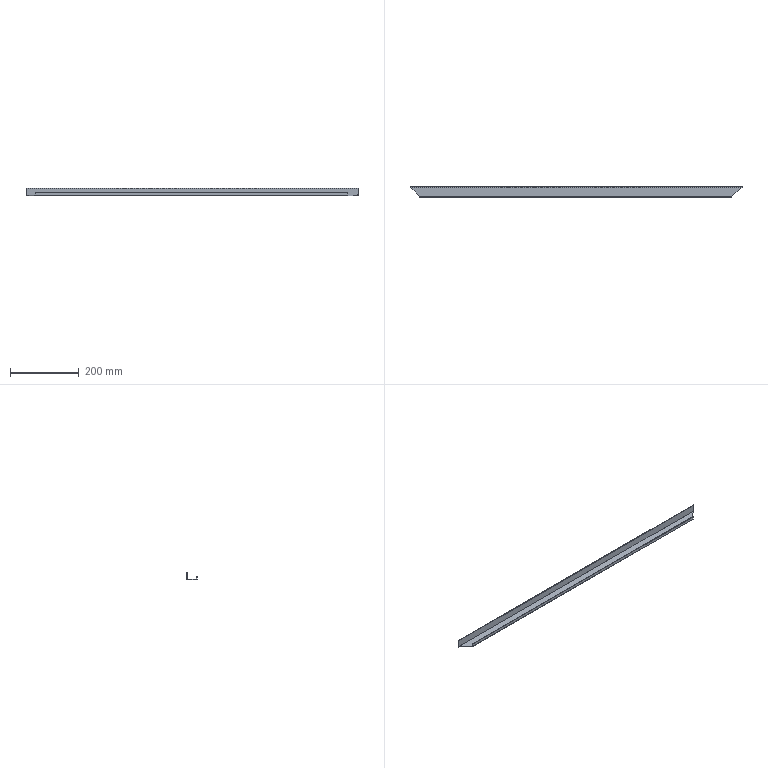Part | STEP file | Rear Closing Plate Door Frame Upper | 1 solid | 34 faces | box 963 x 30 x 22 mm | volume 107174 mm3 | plane 22 | cylinder 10 | spline 2 | commonest cylinder face diameters 0.2 x8 4.2 x2
STEP:
#1=CARTESIAN_POINT('',(-1.351,217.392,2.4));
#2=VERTEX_POINT('',#1);
#3=CARTESIAN_POINT('',(-1.251,217.392,2.3));
#4=VERTEX_POINT('',#3);
#5=CARTESIAN_POINT('',(-1.351,217.392,2.3));
#6=DIRECTION('',(0.,1.,0.));
#7=DIRECTION('',(0.,0.,1.));
#8=AXIS2_PLACEMENT_3D('',#5,#6,#7);
#9=CIRCLE('',#8,0.1);
#10=EDGE_CURVE('',#2,#4,#9,.T.);
#11=ORIENTED_EDGE('',*,*,#10,.F.);
#12=CARTESIAN_POINT('',(-1.351,219.392,2.4));
#13=VERTEX_POINT('',#12);
#14=CARTESIAN_POINT('',(-1.351,-1707.111,2.4));
#15=DIRECTION('',(0.,1.,0.));
#16=VECTOR('',#15,1000.);
#17=LINE('',#14,#16);
#18=EDGE_CURVE('',#2,#13,#17,.T.);
#19=ORIENTED_EDGE('',*,*,#18,.T.);
#20=CARTESIAN_POINT('',(-1.251,219.392,2.3));
#21=VERTEX_POINT('',#20);
#22=CARTESIAN_POINT('',(-1.351,219.392,2.3));
#23=DIRECTION('',(0.,1.,0.));
#24=DIRECTION('',(0.,0.,1.));
#25=AXIS2_PLACEMENT_3D('',#22,#23,#24);
#26=CIRCLE('',#25,0.1);
#27=EDGE_CURVE('',#13,#21,#26,.T.);
#28=ORIENTED_EDGE('',*,*,#27,.T.);
#29=CARTESIAN_POINT('',(-1.251,-1707.111,2.3));
#30=DIRECTION('',(0.,-1.,0.));
#31=VECTOR('',#30,1000.);
#32=LINE('',#29,#31);
#33=EDGE_CURVE('',#21,#4,#32,.T.);
#34=ORIENTED_EDGE('',*,*,#33,.T.);
#35=EDGE_LOOP('',(#11,#19,#28,#34));
#36=FACE_OUTER_BOUND('',#35,.T.);
#37=CARTESIAN_POINT('',(-1.351,-1707.111,2.3));
#38=DIRECTION('',(0.,1.,0.));
#39=DIRECTION('',(0.,0.,1.));
#40=AXIS2_PLACEMENT_3D('',#37,#38,#39);
#41=CYLINDRICAL_SURFACE('',#40,0.1);
#42=ADVANCED_FACE('',(#36),#41,.F.);
#43=CARTESIAN_POINT('',(957.849,217.392,2.4));
#44=VERTEX_POINT('',#43);
#45=CARTESIAN_POINT('',(957.949,217.392,2.3));
#46=VERTEX_POINT('',#45);
#47=CARTESIAN_POINT('',(957.849,217.392,2.3));
#48=DIRECTION('',(0.,1.,0.));
#49=DIRECTION('',(0.,0.,1.));
#50=AXIS2_PLACEMENT_3D('',#47,#48,#49);
#51=CIRCLE('',#50,0.1);
#52=EDGE_CURVE('',#44,#46,#51,.T.);
#53=ORIENTED_EDGE('',*,*,#52,.F.);
#54=CARTESIAN_POINT('',(957.849,219.392,2.4));
#55=VERTEX_POINT('',#54);
#56=CARTESIAN_POINT('',(957.849,-1707.111,2.4));
#57=DIRECTION('',(0.,1.,0.));
#58=VECTOR('',#57,1000.);
#59=LINE('',#56,#58);
#60=EDGE_CURVE('',#44,#55,#59,.T.);
#61=ORIENTED_EDGE('',*,*,#60,.T.);
#62=CARTESIAN_POINT('',(957.949,219.392,2.3));
#63=VERTEX_POINT('',#62);
#64=CARTESIAN_POINT('',(957.849,219.392,2.3));
#65=DIRECTION('',(0.,1.,0.));
#66=DIRECTION('',(0.,0.,1.));
#67=AXIS2_PLACEMENT_3D('',#64,#65,#66);
#68=CIRCLE('',#67,0.1);
#69=EDGE_CURVE('',#55,#63,#68,.T.);
#70=ORIENTED_EDGE('',*,*,#69,.T.);
#71=CARTESIAN_POINT('',(957.949,-1707.111,2.3));
#72=DIRECTION('',(0.,-1.,0.));
#73=VECTOR('',#72,1000.);
#74=LINE('',#71,#73);
#75=EDGE_CURVE('',#63,#46,#74,.T.);
#76=ORIENTED_EDGE('',*,*,#75,.T.);
#77=EDGE_LOOP('',(#53,#61,#70,#76));
#78=FACE_OUTER_BOUND('',#77,.T.);
#79=CARTESIAN_POINT('',(957.849,-1707.111,2.3));
#80=DIRECTION('',(0.,1.,0.));
#81=DIRECTION('',(0.,0.,1.));
#82=AXIS2_PLACEMENT_3D('',#79,#80,#81);
#83=CYLINDRICAL_SURFACE('',#82,0.1);
#84=ADVANCED_FACE('',(#78),#83,.F.);
#85=CARTESIAN_POINT('',(929.749,191.692,2.));
#86=VERTEX_POINT('',#85);
#87=CARTESIAN_POINT('',(929.749,191.492,2.));
#88=VERTEX_POINT('',#87);
#89=CARTESIAN_POINT('',(929.749,0.,2.));
#90=DIRECTION('',(0.,-1.,0.));
#91=VECTOR('',#90,1000.);
#92=LINE('',#89,#91);
#93=EDGE_CURVE('',#86,#88,#92,.T.);
#94=ORIENTED_EDGE('',*,*,#93,.F.);
#95=CARTESIAN_POINT('',(929.949,191.692,2.));
#96=VERTEX_POINT('',#95);
#97=CARTESIAN_POINT('',(929.849,191.692,2.));
#98=DIRECTION('',(0.,0.,-1.));
#99=DIRECTION('',(-1.,0.,0.));
#100=AXIS2_PLACEMENT_3D('',#97,#98,#99);
#101=CIRCLE('',#100,0.1);
#102=EDGE_CURVE('',#86,#96,#101,.T.);
#103=ORIENTED_EDGE('',*,*,#102,.T.);
#104=CARTESIAN_POINT('',(929.949,191.577,2.));
#105=VERTEX_POINT('',#104);
#106=CARTESIAN_POINT('',(929.949,0.,2.));
#107=DIRECTION('',(0.,1.,0.));
#108=VECTOR('',#107,1000.);
#109=LINE('',#106,#108);
#110=EDGE_CURVE('',#105,#96,#109,.T.);
#111=ORIENTED_EDGE('',*,*,#110,.F.);
#112=CARTESIAN_POINT('',(957.641,217.292,2.));
#113=VERTEX_POINT('',#112);
#114=CARTESIAN_POINT('',(957.641,217.292,2.));
#115=DIRECTION('',(-0.7328,-0.6805,0.));
#116=VECTOR('',#115,1000.);
#117=LINE('',#114,#116);
#118=EDGE_CURVE('',#113,#105,#117,.T.);
#119=ORIENTED_EDGE('',*,*,#118,.F.);
#120=CARTESIAN_POINT('',(-1.151,217.292,2.));
#121=VERTEX_POINT('',#120);
#122=CARTESIAN_POINT('',(0.,217.292,2.));
#123=DIRECTION('',(1.,0.,0.));
#124=VECTOR('',#123,1000.);
#125=LINE('',#122,#124);
#126=EDGE_CURVE('',#121,#113,#125,.T.);
#127=ORIENTED_EDGE('',*,*,#126,.F.);
#128=CARTESIAN_POINT('',(24.549,191.592,2.));
#129=VERTEX_POINT('',#128);
#130=CARTESIAN_POINT('',(24.549,191.592,2.));
#131=DIRECTION('',(-0.7071,0.7071,0.));
#132=VECTOR('',#131,1000.);
#133=LINE('',#130,#132);
#134=EDGE_CURVE('',#129,#121,#133,.T.);
#135=ORIENTED_EDGE('',*,*,#134,.F.);
#136=CARTESIAN_POINT('',(24.549,191.692,2.));
#137=VERTEX_POINT('',#136);
#138=CARTESIAN_POINT('',(24.549,0.,2.));
#139=DIRECTION('',(0.,-1.,0.));
#140=VECTOR('',#139,1000.);
#141=LINE('',#138,#140);
#142=EDGE_CURVE('',#137,#129,#141,.T.);
#143=ORIENTED_EDGE('',*,*,#142,.F.);
#144=CARTESIAN_POINT('',(24.749,191.692,2.));
#145=VERTEX_POINT('',#144);
#146=CARTESIAN_POINT('',(24.649,191.692,2.));
#147=DIRECTION('',(0.,0.,-1.));
#148=DIRECTION('',(-1.,0.,0.));
#149=AXIS2_PLACEMENT_3D('',#146,#147,#148);
#150=CIRCLE('',#149,0.1);
#151=EDGE_CURVE('',#137,#145,#150,.T.);
#152=ORIENTED_EDGE('',*,*,#151,.T.);
#153=CARTESIAN_POINT('',(24.749,191.492,2.));
#154=VERTEX_POINT('',#153);
#155=CARTESIAN_POINT('',(24.749,0.,2.));
#156=DIRECTION('',(0.,1.,0.));
#157=VECTOR('',#156,1000.);
#158=LINE('',#155,#157);
#159=EDGE_CURVE('',#154,#145,#158,.T.);
#160=ORIENTED_EDGE('',*,*,#159,.F.);
#161=CARTESIAN_POINT('',(0.,191.492,2.));
#162=DIRECTION('',(-1.,0.,0.));
#163=VECTOR('',#162,1000.);
#164=LINE('',#161,#163);
#165=EDGE_CURVE('',#88,#154,#164,.T.);
#166=ORIENTED_EDGE('',*,*,#165,.F.);
#167=EDGE_LOOP('',(#94,#103,#111,#119,#127,#135,#143,#152,#160,#166));
#168=FACE_OUTER_BOUND('',#167,.T.);
#169=CARTESIAN_POINT('',(0.,0.,2.));
#170=DIRECTION('',(0.,0.,-1.));
#171=DIRECTION('',(-1.,0.,0.));
#172=AXIS2_PLACEMENT_3D('',#169,#170,#171);
#173=PLANE('',#172);
#174=ADVANCED_FACE('',(#168),#173,.F.);
#175=CARTESIAN_POINT('',(24.749,191.392,2.1));
#176=VERTEX_POINT('',#175);
#177=CARTESIAN_POINT('',(24.749,191.492,2.1));
#178=DIRECTION('',(1.,0.,0.));
#179=DIRECTION('',(0.,0.,-1.));
#180=AXIS2_PLACEMENT_3D('',#177,#178,#179);
#181=CIRCLE('',#180,0.1);
#182=EDGE_CURVE('',#176,#154,#181,.T.);
#183=ORIENTED_EDGE('',*,*,#182,.F.);
#184=CARTESIAN_POINT('',(929.749,191.392,2.1));
#185=VERTEX_POINT('',#184);
#186=CARTESIAN_POINT('',(-939.217,191.392,2.1));
#187=DIRECTION('',(-1.,0.,0.));
#188=VECTOR('',#187,1000.);
#189=LINE('',#186,#188);
#190=EDGE_CURVE('',#185,#176,#189,.T.);
#191=ORIENTED_EDGE('',*,*,#190,.F.);
#192=CARTESIAN_POINT('',(929.749,191.492,2.1));
#193=DIRECTION('',(-1.,0.,0.));
#194=DIRECTION('',(0.,0.,-1.));
#195=AXIS2_PLACEMENT_3D('',#192,#193,#194);
#196=CIRCLE('',#195,0.1);
#197=EDGE_CURVE('',#88,#185,#196,.T.);
#198=ORIENTED_EDGE('',*,*,#197,.F.);
#199=ORIENTED_EDGE('',*,*,#165,.T.);
#200=EDGE_LOOP('',(#183,#191,#198,#199));
#201=FACE_OUTER_BOUND('',#200,.T.);
#202=CARTESIAN_POINT('',(-939.217,191.492,2.1));
#203=DIRECTION('',(1.,0.,0.));
#204=DIRECTION('',(0.,0.,-1.));
#205=AXIS2_PLACEMENT_3D('',#202,#203,#204);
#206=CYLINDRICAL_SURFACE('',#205,0.1);
#207=ADVANCED_FACE('',(#201),#206,.F.);
#208=CARTESIAN_POINT('',(957.641,217.292,0.));
#209=VERTEX_POINT('',#208);
#210=CARTESIAN_POINT('',(957.641,217.292,1918.279));
#211=DIRECTION('',(0.,0.,1.));
#212=VECTOR('',#211,1000.);
#213=LINE('',#210,#212);
#214=EDGE_CURVE('',#209,#113,#213,.T.);
#215=ORIENTED_EDGE('',*,*,#214,.T.);
#216=ORIENTED_EDGE('',*,*,#118,.T.);
#217=CARTESIAN_POINT('',(929.949,191.577,0.));
#218=VERTEX_POINT('',#217);
#219=CARTESIAN_POINT('',(929.949,191.577,1918.279));
#220=DIRECTION('',(0.,0.,-1.));
#221=VECTOR('',#220,1000.);
#222=LINE('',#219,#221);
#223=EDGE_CURVE('',#105,#218,#222,.T.);
#224=ORIENTED_EDGE('',*,*,#223,.T.);
#225=CARTESIAN_POINT('',(335.053,-360.826,0.));
#226=DIRECTION('',(0.7328,0.6805,0.));
#227=VECTOR('',#226,1000.);
#228=LINE('',#225,#227);
#229=EDGE_CURVE('',#218,#209,#228,.T.);
#230=ORIENTED_EDGE('',*,*,#229,.T.);
#231=EDGE_LOOP('',(#215,#216,#224,#230));
#232=FACE_OUTER_BOUND('',#231,.T.);
#233=CARTESIAN_POINT('',(335.053,-360.826,1918.279));
#234=DIRECTION('',(0.6805,-0.7328,0.));
#235=DIRECTION('',(0.7328,0.6805,0.));
#236=AXIS2_PLACEMENT_3D('',#233,#234,#235);
#237=PLANE('',#236);
#238=ADVANCED_FACE('',(#232),#237,.T.);
#239=CARTESIAN_POINT('',(957.749,217.304,2.001));
#240=VERTEX_POINT('',#239);
#241=CARTESIAN_POINT('',(957.749,217.304,2.001));
#242=CARTESIAN_POINT('',(957.713,217.3,2.));
#243=CARTESIAN_POINT('',(957.677,217.296,2.));
#244=CARTESIAN_POINT('',(957.641,217.292,2.));
#245=B_SPLINE_CURVE_WITH_KNOTS('',3,(#241,#242,#243,#244),.UNSPECIFIED.,.F.,.F.,(4,4),(0.,1.),.UNSPECIFIED.);
#246=EDGE_CURVE('',#240,#113,#245,.T.);
#247=ORIENTED_EDGE('',*,*,#246,.F.);
#248=CARTESIAN_POINT('',(957.749,217.392,2.1));
#249=VERTEX_POINT('',#248);
#250=CARTESIAN_POINT('',(957.749,217.292,2.1));
#251=DIRECTION('',(-1.,0.,0.));
#252=DIRECTION('',(0.,0.,1.));
#253=AXIS2_PLACEMENT_3D('',#250,#251,#252);
#254=CIRCLE('',#253,0.1);
#255=EDGE_CURVE('',#249,#240,#254,.T.);
#256=ORIENTED_EDGE('',*,*,#255,.F.);
#257=CARTESIAN_POINT('',(-1.251,217.392,2.1));
#258=VERTEX_POINT('',#257);
#259=CARTESIAN_POINT('',(1922.392,217.392,2.1));
#260=DIRECTION('',(1.,0.,0.));
#261=VECTOR('',#260,1000.);
#262=LINE('',#259,#261);
#263=EDGE_CURVE('',#258,#249,#262,.T.);
#264=ORIENTED_EDGE('',*,*,#263,.F.);
#265=CARTESIAN_POINT('',(-1.251,217.304,2.001));
#266=VERTEX_POINT('',#265);
#267=CARTESIAN_POINT('',(-1.251,217.292,2.1));
#268=DIRECTION('',(1.,0.,0.));
#269=DIRECTION('',(0.,0.,1.));
#270=AXIS2_PLACEMENT_3D('',#267,#268,#269);
#271=CIRCLE('',#270,0.1);
#272=EDGE_CURVE('',#266,#258,#271,.T.);
#273=ORIENTED_EDGE('',*,*,#272,.F.);
#274=CARTESIAN_POINT('',(-1.151,217.292,2.));
#275=CARTESIAN_POINT('',(-1.184,217.296,2.));
#276=CARTESIAN_POINT('',(-1.218,217.3,2.));
#277=CARTESIAN_POINT('',(-1.251,217.304,2.001));
#278=B_SPLINE_CURVE_WITH_KNOTS('',3,(#274,#275,#276,#277),.UNSPECIFIED.,.F.,.F.,(4,4),(0.,1.),.UNSPECIFIED.);
#279=EDGE_CURVE('',#121,#266,#278,.T.);
#280=ORIENTED_EDGE('',*,*,#279,.F.);
#281=ORIENTED_EDGE('',*,*,#126,.T.);
#282=EDGE_LOOP('',(#247,#256,#264,#273,#280,#281));
#283=FACE_OUTER_BOUND('',#282,.T.);
#284=CARTESIAN_POINT('',(1922.392,217.292,2.1));
#285=DIRECTION('',(-1.,0.,0.));
#286=DIRECTION('',(0.,0.,1.));
#287=AXIS2_PLACEMENT_3D('',#284,#285,#286);
#288=CYLINDRICAL_SURFACE('',#287,0.1);
#289=ADVANCED_FACE('',(#283),#288,.F.);
#290=CARTESIAN_POINT('',(24.549,191.592,0.));
#291=VERTEX_POINT('',#290);
#292=CARTESIAN_POINT('',(24.549,191.592,1918.279));
#293=DIRECTION('',(0.,0.,1.));
#294=VECTOR('',#293,1000.);
#295=LINE('',#292,#294);
#296=EDGE_CURVE('',#291,#129,#295,.T.);
#297=ORIENTED_EDGE('',*,*,#296,.T.);
#298=ORIENTED_EDGE('',*,*,#134,.T.);
#299=CARTESIAN_POINT('',(-1.151,217.292,0.));
#300=VERTEX_POINT('',#299);
#301=CARTESIAN_POINT('',(-1.151,217.292,1918.279));
#302=DIRECTION('',(0.,0.,-1.));
#303=VECTOR('',#302,1000.);
#304=LINE('',#301,#303);
#305=EDGE_CURVE('',#121,#300,#304,.T.);
#306=ORIENTED_EDGE('',*,*,#305,.T.);
#307=CARTESIAN_POINT('',(108.07,108.07,0.));
#308=DIRECTION('',(0.7071,-0.7071,0.));
#309=VECTOR('',#308,1000.);
#310=LINE('',#307,#309);
#311=EDGE_CURVE('',#300,#291,#310,.T.);
#312=ORIENTED_EDGE('',*,*,#311,.T.);
#313=EDGE_LOOP('',(#297,#298,#306,#312));
#314=FACE_OUTER_BOUND('',#313,.T.);
#315=CARTESIAN_POINT('',(108.07,108.07,1918.279));
#316=DIRECTION('',(-0.7071,-0.7071,0.));
#317=DIRECTION('',(0.7071,-0.7071,0.));
#318=AXIS2_PLACEMENT_3D('',#315,#316,#317);
#319=PLANE('',#318);
#320=ADVANCED_FACE('',(#314),#319,.T.);
#321=ORIENTED_EDGE('',*,*,#190,.T.);
#322=CARTESIAN_POINT('',(24.749,191.392,10.));
#323=VERTEX_POINT('',#322);
#324=CARTESIAN_POINT('',(24.749,191.392,22.));
#325=DIRECTION('',(0.,0.,-1.));
#326=VECTOR('',#325,1000.);
#327=LINE('',#324,#326);
#328=EDGE_CURVE('',#323,#176,#327,.T.);
#329=ORIENTED_EDGE('',*,*,#328,.F.);
#330=CARTESIAN_POINT('',(929.749,191.392,10.));
#331=VERTEX_POINT('',#330);
#332=CARTESIAN_POINT('',(26.749,191.392,10.));
#333=DIRECTION('',(-1.,0.,0.));
#334=VECTOR('',#333,1000.);
#335=LINE('',#332,#334);
#336=EDGE_CURVE('',#331,#323,#335,.T.);
#337=ORIENTED_EDGE('',*,*,#336,.F.);
#338=CARTESIAN_POINT('',(929.749,191.392,22.));
#339=DIRECTION('',(0.,0.,1.));
#340=VECTOR('',#339,1000.);
#341=LINE('',#338,#340);
#342=EDGE_CURVE('',#185,#331,#341,.T.);
#343=ORIENTED_EDGE('',*,*,#342,.F.);
#344=EDGE_LOOP('',(#321,#329,#337,#343));
#345=FACE_OUTER_BOUND('',#344,.T.);
#346=CARTESIAN_POINT('',(26.749,191.392,22.));
#347=DIRECTION('',(0.,-1.,0.));
#348=DIRECTION('',(0.,0.,-1.));
#349=AXIS2_PLACEMENT_3D('',#346,#347,#348);
#350=PLANE('',#349);
#351=ADVANCED_FACE('',(#345),#350,.F.);
#352=ORIENTED_EDGE('',*,*,#214,.F.);
#353=CARTESIAN_POINT('',(957.749,217.541,0.01486));
#354=VERTEX_POINT('',#353);
#355=CARTESIAN_POINT('',(957.749,217.541,0.01486));
#356=CARTESIAN_POINT('',(957.713,217.458,0.004966));
#357=CARTESIAN_POINT('',(957.677,217.375,0.));
#358=CARTESIAN_POINT('',(957.641,217.292,0.));
#359=B_SPLINE_CURVE_WITH_KNOTS('',3,(#355,#356,#357,#358),.UNSPECIFIED.,.F.,.F.,(4,4),(0.,1.),.UNSPECIFIED.);
#360=EDGE_CURVE('',#354,#209,#359,.T.);
#361=ORIENTED_EDGE('',*,*,#360,.F.);
#362=CARTESIAN_POINT('',(957.749,217.422,1.008));
#363=DIRECTION('',(0.,-0.1188,0.9929));
#364=VECTOR('',#363,1000.);
#365=LINE('',#362,#364);
#366=EDGE_CURVE('',#354,#240,#365,.T.);
#367=ORIENTED_EDGE('',*,*,#366,.T.);
#368=ORIENTED_EDGE('',*,*,#246,.T.);
#369=EDGE_LOOP('',(#352,#361,#367,#368));
#370=FACE_OUTER_BOUND('',#369,.T.);
#371=CARTESIAN_POINT('',(957.749,217.541,0.01486));
#372=CARTESIAN_POINT('',(957.713,217.458,0.004966));
#373=CARTESIAN_POINT('',(957.677,217.375,0.));
#374=CARTESIAN_POINT('',(957.641,217.292,0.));
#375=CARTESIAN_POINT('',(957.749,217.304,2.001));
#376=CARTESIAN_POINT('',(957.713,217.3,2.));
#377=CARTESIAN_POINT('',(957.677,217.296,2.));
#378=CARTESIAN_POINT('',(957.641,217.292,2.));
#379=B_SPLINE_SURFACE_WITH_KNOTS('',1,3,((#371,#372,#373,#374),(#375,#376,#377,#378)),.UNSPECIFIED.,.F.,.F.,.F.,(2,2),(4,4),(0.,1.),(0.,1.),.UNSPECIFIED.);
#380=ADVANCED_FACE('',(#370),#379,.T.);
#381=CARTESIAN_POINT('',(929.949,191.692,0.));
#382=VERTEX_POINT('',#381);
#383=CARTESIAN_POINT('',(929.949,0.,0.));
#384=DIRECTION('',(0.,1.,0.));
#385=VECTOR('',#384,1000.);
#386=LINE('',#383,#385);
#387=EDGE_CURVE('',#218,#382,#386,.T.);
#388=ORIENTED_EDGE('',*,*,#387,.T.);
#389=CARTESIAN_POINT('',(929.749,191.692,0.));
#390=VERTEX_POINT('',#389);
#391=CARTESIAN_POINT('',(929.849,191.692,0.));
#392=DIRECTION('',(0.,0.,1.));
#393=DIRECTION('',(-1.,0.,0.));
#394=AXIS2_PLACEMENT_3D('',#391,#392,#393);
#395=CIRCLE('',#394,0.1);
#396=EDGE_CURVE('',#382,#390,#395,.T.);
#397=ORIENTED_EDGE('',*,*,#396,.T.);
#398=CARTESIAN_POINT('',(929.749,191.492,0.));
#399=VERTEX_POINT('',#398);
#400=CARTESIAN_POINT('',(929.749,0.,0.));
#401=DIRECTION('',(0.,1.,0.));
#402=VECTOR('',#401,1000.);
#403=LINE('',#400,#402);
#404=EDGE_CURVE('',#399,#390,#403,.T.);
#405=ORIENTED_EDGE('',*,*,#404,.F.);
#406=CARTESIAN_POINT('',(24.749,191.492,0.));
#407=VERTEX_POINT('',#406);
#408=CARTESIAN_POINT('',(0.,191.492,0.));
#409=DIRECTION('',(-1.,0.,0.));
#410=VECTOR('',#409,1000.);
#411=LINE('',#408,#410);
#412=EDGE_CURVE('',#399,#407,#411,.T.);
#413=ORIENTED_EDGE('',*,*,#412,.T.);
#414=CARTESIAN_POINT('',(24.749,191.692,0.));
#415=VERTEX_POINT('',#414);
#416=CARTESIAN_POINT('',(24.749,0.,0.));
#417=DIRECTION('',(0.,-1.,0.));
#418=VECTOR('',#417,1000.);
#419=LINE('',#416,#418);
#420=EDGE_CURVE('',#415,#407,#419,.T.);
#421=ORIENTED_EDGE('',*,*,#420,.F.);
#422=CARTESIAN_POINT('',(24.549,191.692,0.));
#423=VERTEX_POINT('',#422);
#424=CARTESIAN_POINT('',(24.649,191.692,0.));
#425=DIRECTION('',(0.,0.,1.));
#426=DIRECTION('',(-1.,0.,0.));
#427=AXIS2_PLACEMENT_3D('',#424,#425,#426);
#428=CIRCLE('',#427,0.1);
#429=EDGE_CURVE('',#415,#423,#428,.T.);
#430=ORIENTED_EDGE('',*,*,#429,.T.);
#431=CARTESIAN_POINT('',(24.549,0.,0.));
#432=DIRECTION('',(0.,-1.,0.));
#433=VECTOR('',#432,1000.);
#434=LINE('',#431,#433);
#435=EDGE_CURVE('',#423,#291,#434,.T.);
#436=ORIENTED_EDGE('',*,*,#435,.T.);
#437=ORIENTED_EDGE('',*,*,#311,.F.);
#438=CARTESIAN_POINT('',(0.,217.292,0.));
#439=DIRECTION('',(1.,0.,0.));
#440=VECTOR('',#439,1000.);
#441=LINE('',#438,#440);
#442=EDGE_CURVE('',#300,#209,#441,.T.);
#443=ORIENTED_EDGE('',*,*,#442,.T.);
#444=ORIENTED_EDGE('',*,*,#229,.F.);
#445=EDGE_LOOP('',(#388,#397,#405,#413,#421,#430,#436,#437,#443,#444));
#446=FACE_OUTER_BOUND('',#445,.T.);
#447=CARTESIAN_POINT('',(0.,0.,0.));
#448=DIRECTION('',(0.,0.,-1.));
#449=DIRECTION('',(-1.,0.,0.));
#450=AXIS2_PLACEMENT_3D('',#447,#448,#449);
#451=PLANE('',#450);
#452=ADVANCED_FACE('',(#446),#451,.T.);
#453=ORIENTED_EDGE('',*,*,#223,.F.);
#454=ORIENTED_EDGE('',*,*,#110,.T.);
#455=CARTESIAN_POINT('',(929.949,191.692,1918.279));
#456=DIRECTION('',(0.,0.,-1.));
#457=VECTOR('',#456,1000.);
#458=LINE('',#455,#457);
#459=EDGE_CURVE('',#96,#382,#458,.T.);
#460=ORIENTED_EDGE('',*,*,#459,.T.);
#461=ORIENTED_EDGE('',*,*,#387,.F.);
#462=EDGE_LOOP('',(#453,#454,#460,#461));
#463=FACE_OUTER_BOUND('',#462,.T.);
#464=CARTESIAN_POINT('',(929.949,0.,1918.279));
#465=DIRECTION('',(-1.,0.,0.));
#466=DIRECTION('',(0.,0.,1.));
#467=AXIS2_PLACEMENT_3D('',#464,#465,#466);
#468=PLANE('',#467);
#469=ADVANCED_FACE('',(#463),#468,.T.);
#470=CARTESIAN_POINT('',(-1.451,217.392,2.3));
#471=VERTEX_POINT('',#470);
#472=CARTESIAN_POINT('',(-1.351,217.392,2.3));
#473=DIRECTION('',(0.,1.,0.));
#474=DIRECTION('',(0.,0.,1.));
#475=AXIS2_PLACEMENT_3D('',#472,#473,#474);
#476=CIRCLE('',#475,0.1);
#477=EDGE_CURVE('',#471,#2,#476,.T.);
#478=ORIENTED_EDGE('',*,*,#477,.T.);
#479=ORIENTED_EDGE('',*,*,#10,.T.);
#480=CARTESIAN_POINT('',(-1.251,217.392,22.));
#481=DIRECTION('',(0.,0.,-1.));
#482=VECTOR('',#481,1000.);
#483=LINE('',#480,#482);
#484=EDGE_CURVE('',#4,#258,#483,.T.);
#485=ORIENTED_EDGE('',*,*,#484,.T.);
#486=ORIENTED_EDGE('',*,*,#263,.T.);
#487=CARTESIAN_POINT('',(957.749,217.392,2.3));
#488=VERTEX_POINT('',#487);
#489=CARTESIAN_POINT('',(957.749,217.392,22.));
#490=DIRECTION('',(0.,0.,1.));
#491=VECTOR('',#490,1000.);
#492=LINE('',#489,#491);
#493=EDGE_CURVE('',#249,#488,#492,.T.);
#494=ORIENTED_EDGE('',*,*,#493,.T.);
#495=CARTESIAN_POINT('',(957.849,217.392,2.3));
#496=DIRECTION('',(0.,1.,0.));
#497=DIRECTION('',(0.,0.,1.));
#498=AXIS2_PLACEMENT_3D('',#495,#496,#497);
#499=CIRCLE('',#498,0.1);
#500=EDGE_CURVE('',#488,#44,#499,.T.);
#501=ORIENTED_EDGE('',*,*,#500,.T.);
#502=ORIENTED_EDGE('',*,*,#52,.T.);
#503=CARTESIAN_POINT('',(957.949,217.392,0.));
#504=VERTEX_POINT('',#503);
#505=CARTESIAN_POINT('',(957.949,217.392,22.));
#506=DIRECTION('',(0.,0.,-1.));
#507=VECTOR('',#506,1000.);
#508=LINE('',#505,#507);
#509=EDGE_CURVE('',#46,#504,#508,.T.);
#510=ORIENTED_EDGE('',*,*,#509,.T.);
#511=CARTESIAN_POINT('',(959.749,217.392,0.));
#512=VERTEX_POINT('',#511);
#513=CARTESIAN_POINT('',(-3.251,217.392,0.));
#514=DIRECTION('',(1.,0.,0.));
#515=VECTOR('',#514,1000.);
#516=LINE('',#513,#515);
#517=EDGE_CURVE('',#504,#512,#516,.T.);
#518=ORIENTED_EDGE('',*,*,#517,.T.);
#519=CARTESIAN_POINT('',(959.749,217.392,22.));
#520=VERTEX_POINT('',#519);
#521=CARTESIAN_POINT('',(959.749,217.392,22.));
#522=DIRECTION('',(0.,0.,1.));
#523=VECTOR('',#522,1000.);
#524=LINE('',#521,#523);
#525=EDGE_CURVE('',#512,#520,#524,.T.);
#526=ORIENTED_EDGE('',*,*,#525,.T.);
#527=CARTESIAN_POINT('',(-3.251,217.392,22.));
#528=VERTEX_POINT('',#527);
#529=CARTESIAN_POINT('',(-3.251,217.392,22.));
#530=DIRECTION('',(-1.,0.,0.));
#531=VECTOR('',#530,1000.);
#532=LINE('',#529,#531);
#533=EDGE_CURVE('',#520,#528,#532,.T.);
#534=ORIENTED_EDGE('',*,*,#533,.T.);
#535=CARTESIAN_POINT('',(-3.251,217.392,0.));
#536=VERTEX_POINT('',#535);
#537=CARTESIAN_POINT('',(-3.251,217.392,22.));
#538=DIRECTION('',(0.,0.,-1.));
#539=VECTOR('',#538,1000.);
#540=LINE('',#537,#539);
#541=EDGE_CURVE('',#528,#536,#540,.T.);
#542=ORIENTED_EDGE('',*,*,#541,.T.);
#543=CARTESIAN_POINT('',(-1.451,217.392,0.));
#544=VERTEX_POINT('',#543);
#545=CARTESIAN_POINT('',(-3.251,217.392,0.));
#546=DIRECTION('',(1.,0.,0.));
#547=VECTOR('',#546,1000.);
#548=LINE('',#545,#547);
#549=EDGE_CURVE('',#536,#544,#548,.T.);
#550=ORIENTED_EDGE('',*,*,#549,.T.);
#551=CARTESIAN_POINT('',(-1.451,217.392,22.));
#552=DIRECTION('',(0.,0.,1.));
#553=VECTOR('',#552,1000.);
#554=LINE('',#551,#553);
#555=EDGE_CURVE('',#544,#471,#554,.T.);
#556=ORIENTED_EDGE('',*,*,#555,.T.);
#557=EDGE_LOOP('',(#478,#479,#485,#486,#494,#501,#502,#510,#518,#526,#534,#542,#550,#556));
#558=FACE_OUTER_BOUND('',#557,.T.);
#559=CARTESIAN_POINT('',(-3.251,217.392,22.));
#560=DIRECTION('',(0.,-1.,0.));
#561=DIRECTION('',(0.,0.,-1.));
#562=AXIS2_PLACEMENT_3D('',#559,#560,#561);
#563=PLANE('',#562);
#564=ADVANCED_FACE('',(#558),#563,.T.);
#565=CARTESIAN_POINT('',(24.549,191.692,1918.279));
#566=DIRECTION('',(0.,0.,1.));
#567=VECTOR('',#566,1000.);
#568=LINE('',#565,#567);
#569=EDGE_CURVE('',#423,#137,#568,.T.);
#570=ORIENTED_EDGE('',*,*,#569,.T.);
#571=ORIENTED_EDGE('',*,*,#142,.T.);
#572=ORIENTED_EDGE('',*,*,#296,.F.);
#573=ORIENTED_EDGE('',*,*,#435,.F.);
#574=EDGE_LOOP('',(#570,#571,#572,#573));
#575=FACE_OUTER_BOUND('',#574,.T.);
#576=CARTESIAN_POINT('',(24.549,0.,1918.279));
#577=DIRECTION('',(1.,0.,0.));
#578=DIRECTION('',(0.,0.,-1.));
#579=AXIS2_PLACEMENT_3D('',#576,#577,#578);
#580=PLANE('',#579);
#581=ADVANCED_FACE('',(#575),#580,.T.);
#582=CARTESIAN_POINT('',(-1.251,217.541,0.01486));
#583=VERTEX_POINT('',#582);
#584=CARTESIAN_POINT('',(-1.251,217.541,0.01486));
#585=CARTESIAN_POINT('',(-1.218,217.458,0.004966));
#586=CARTESIAN_POINT('',(-1.184,217.375,0.));
#587=CARTESIAN_POINT('',(-1.151,217.292,0.));
#588=B_SPLINE_CURVE_WITH_KNOTS('',3,(#584,#585,#586,#587),.UNSPECIFIED.,.F.,.F.,(4,4),(0.,1.),.UNSPECIFIED.);
#589=EDGE_CURVE('',#583,#300,#588,.T.);
#590=ORIENTED_EDGE('',*,*,#589,.T.);
#591=ORIENTED_EDGE('',*,*,#305,.F.);
#592=ORIENTED_EDGE('',*,*,#279,.T.);
#593=CARTESIAN_POINT('',(-1.251,217.422,1.008));
#594=DIRECTION('',(0.,0.1188,-0.9929));
#595=VECTOR('',#594,1000.);
#596=LINE('',#593,#595);
#597=EDGE_CURVE('',#266,#583,#596,.T.);
#598=ORIENTED_EDGE('',*,*,#597,.T.);
#599=EDGE_LOOP('',(#590,#591,#592,#598));
#600=FACE_OUTER_BOUND('',#599,.T.);
#601=CARTESIAN_POINT('',(-1.151,217.292,0.));
#602=CARTESIAN_POINT('',(-1.184,217.375,0.));
#603=CARTESIAN_POINT('',(-1.218,217.458,0.004966));
#604=CARTESIAN_POINT('',(-1.251,217.541,0.01486));
#605=CARTESIAN_POINT('',(-1.151,217.292,2.));
#606=CARTESIAN_POINT('',(-1.184,217.296,2.));
#607=CARTESIAN_POINT('',(-1.218,217.3,2.));
#608=CARTESIAN_POINT('',(-1.251,217.304,2.001));
#609=B_SPLINE_SURFACE_WITH_KNOTS('',1,3,((#601,#602,#603,#604),(#605,#606,#607,#608)),.UNSPECIFIED.,.F.,.F.,.F.,(2,2),(4,4),(0.,1.),(0.,1.),.UNSPECIFIED.);
#610=ADVANCED_FACE('',(#600),#609,.T.);
#611=CARTESIAN_POINT('',(929.749,189.392,2.1));
#612=VERTEX_POINT('',#611);
#613=CARTESIAN_POINT('',(929.749,189.392,10.));
#614=VERTEX_POINT('',#613);
#615=CARTESIAN_POINT('',(929.749,189.392,22.));
#616=DIRECTION('',(0.,0.,1.));
#617=VECTOR('',#616,1000.);
#618=LINE('',#615,#617);
#619=EDGE_CURVE('',#612,#614,#618,.T.);
#620=ORIENTED_EDGE('',*,*,#619,.F.);
#621=CARTESIAN_POINT('',(929.749,191.492,2.1));
#622=DIRECTION('',(-1.,0.,0.));
#623=DIRECTION('',(0.,0.,-1.));
#624=AXIS2_PLACEMENT_3D('',#621,#622,#623);
#625=CIRCLE('',#624,2.1);
#626=EDGE_CURVE('',#399,#612,#625,.T.);
#627=ORIENTED_EDGE('',*,*,#626,.F.);
#628=ORIENTED_EDGE('',*,*,#404,.T.);
#629=CARTESIAN_POINT('',(929.749,191.692,1918.279));
#630=DIRECTION('',(0.,0.,1.));
#631=VECTOR('',#630,1000.);
#632=LINE('',#629,#631);
#633=EDGE_CURVE('',#390,#86,#632,.T.);
#634=ORIENTED_EDGE('',*,*,#633,.T.);
#635=ORIENTED_EDGE('',*,*,#93,.T.);
#636=ORIENTED_EDGE('',*,*,#197,.T.);
#637=ORIENTED_EDGE('',*,*,#342,.T.);
#638=CARTESIAN_POINT('',(929.749,1999.461,10.));
#639=DIRECTION('',(0.,1.,0.));
#640=VECTOR('',#639,1000.);
#641=LINE('',#638,#640);
#642=EDGE_CURVE('',#614,#331,#641,.T.);
#643=ORIENTED_EDGE('',*,*,#642,.F.);
#644=EDGE_LOOP('',(#620,#627,#628,#634,#635,#636,#637,#643));
#645=FACE_OUTER_BOUND('',#644,.T.);
#646=CARTESIAN_POINT('',(929.749,1999.461,22.));
#647=DIRECTION('',(-1.,0.,0.));
#648=DIRECTION('',(0.,0.,1.));
#649=AXIS2_PLACEMENT_3D('',#646,#647,#648);
#650=PLANE('',#649);
#651=ADVANCED_FACE('',(#645),#650,.F.);
#652=CARTESIAN_POINT('',(24.749,189.392,10.));
#653=VERTEX_POINT('',#652);
#654=CARTESIAN_POINT('',(24.749,1999.461,10.));
#655=DIRECTION('',(0.,1.,0.));
#656=VECTOR('',#655,1000.);
#657=LINE('',#654,#656);
#658=EDGE_CURVE('',#653,#323,#657,.T.);
#659=ORIENTED_EDGE('',*,*,#658,.T.);
#660=ORIENTED_EDGE('',*,*,#328,.T.);
#661=ORIENTED_EDGE('',*,*,#182,.T.);
#662=ORIENTED_EDGE('',*,*,#159,.T.);
#663=CARTESIAN_POINT('',(24.749,191.692,1918.279));
#664=DIRECTION('',(0.,0.,-1.));
#665=VECTOR('',#664,1000.);
#666=LINE('',#663,#665);
#667=EDGE_CURVE('',#145,#415,#666,.T.);
#668=ORIENTED_EDGE('',*,*,#667,.T.);
#669=ORIENTED_EDGE('',*,*,#420,.T.);
#670=CARTESIAN_POINT('',(24.749,189.392,2.1));
#671=VERTEX_POINT('',#670);
#672=CARTESIAN_POINT('',(24.749,191.492,2.1));
#673=DIRECTION('',(1.,0.,0.));
#674=DIRECTION('',(0.,0.,-1.));
#675=AXIS2_PLACEMENT_3D('',#672,#673,#674);
#676=CIRCLE('',#675,2.1);
#677=EDGE_CURVE('',#671,#407,#676,.T.);
#678=ORIENTED_EDGE('',*,*,#677,.F.);
#679=CARTESIAN_POINT('',(24.749,189.392,22.));
#680=DIRECTION('',(0.,0.,1.));
#681=VECTOR('',#680,1000.);
#682=LINE('',#679,#681);
#683=EDGE_CURVE('',#671,#653,#682,.T.);
#684=ORIENTED_EDGE('',*,*,#683,.T.);
#685=EDGE_LOOP('',(#659,#660,#661,#662,#668,#669,#678,#684));
#686=FACE_OUTER_BOUND('',#685,.T.);
#687=CARTESIAN_POINT('',(24.749,1999.461,22.));
#688=DIRECTION('',(-1.,0.,0.));
#689=DIRECTION('',(0.,0.,1.));
#690=AXIS2_PLACEMENT_3D('',#687,#688,#689);
#691=PLANE('',#690);
#692=ADVANCED_FACE('',(#686),#691,.T.);
#693=ORIENTED_EDGE('',*,*,#642,.T.);
#694=ORIENTED_EDGE('',*,*,#336,.T.);
#695=ORIENTED_EDGE('',*,*,#658,.F.);
#696=CARTESIAN_POINT('',(24.749,189.392,10.));
#697=DIRECTION('',(1.,0.,0.));
#698=VECTOR('',#697,1000.);
#699=LINE('',#696,#698);
#700=EDGE_CURVE('',#653,#614,#699,.T.);
#701=ORIENTED_EDGE('',*,*,#700,.T.);
#702=EDGE_LOOP('',(#693,#694,#695,#701));
#703=FACE_OUTER_BOUND('',#702,.T.);
#704=CARTESIAN_POINT('',(24.749,1999.461,10.));
#705=DIRECTION('',(0.,0.,1.));
#706=DIRECTION('',(1.,0.,0.));
#707=AXIS2_PLACEMENT_3D('',#704,#705,#706);
#708=PLANE('',#707);
#709=ADVANCED_FACE('',(#703),#708,.T.);
#710=ORIENTED_EDGE('',*,*,#366,.F.);
#711=CARTESIAN_POINT('',(957.749,219.392,2.1));
#712=VERTEX_POINT('',#711);
#713=CARTESIAN_POINT('',(957.749,217.292,2.1));
#714=DIRECTION('',(1.,0.,0.));
#715=DIRECTION('',(0.,0.,1.));
#716=AXIS2_PLACEMENT_3D('',#713,#714,#715);
#717=CIRCLE('',#716,2.1);
#718=EDGE_CURVE('',#354,#712,#717,.T.);
#719=ORIENTED_EDGE('',*,*,#718,.T.);
#720=CARTESIAN_POINT('',(957.749,219.392,2.3));
#721=VERTEX_POINT('',#720);
#722=CARTESIAN_POINT('',(957.749,219.392,22.));
#723=DIRECTION('',(0.,0.,-1.));
#724=VECTOR('',#723,1000.);
#725=LINE('',#722,#724);
#726=EDGE_CURVE('',#721,#712,#725,.T.);
#727=ORIENTED_EDGE('',*,*,#726,.F.);
#728=CARTESIAN_POINT('',(957.749,-1707.111,2.3));
#729=DIRECTION('',(0.,1.,0.));
#730=VECTOR('',#729,1000.);
#731=LINE('',#728,#730);
#732=EDGE_CURVE('',#488,#721,#731,.T.);
#733=ORIENTED_EDGE('',*,*,#732,.F.);
#734=ORIENTED_EDGE('',*,*,#493,.F.);
#735=ORIENTED_EDGE('',*,*,#255,.T.);
#736=EDGE_LOOP('',(#710,#719,#727,#733,#734,#735));
#737=FACE_OUTER_BOUND('',#736,.T.);
#738=CARTESIAN_POINT('',(957.749,217.292,2.1));
#739=DIRECTION('',(1.,0.,0.));
#740=DIRECTION('',(0.,0.,-1.));
#741=AXIS2_PLACEMENT_3D('',#738,#739,#740);
#742=PLANE('',#741);
#743=ADVANCED_FACE('',(#737),#742,.T.);
#744=ORIENTED_EDGE('',*,*,#718,.F.);
#745=ORIENTED_EDGE('',*,*,#360,.T.);
#746=ORIENTED_EDGE('',*,*,#442,.F.);
#747=ORIENTED_EDGE('',*,*,#589,.F.);
#748=CARTESIAN_POINT('',(-1.251,219.392,2.1));
#749=VERTEX_POINT('',#748);
#750=CARTESIAN_POINT('',(-1.251,217.292,2.1));
#751=DIRECTION('',(1.,0.,0.));
#752=DIRECTION('',(0.,0.,1.));
#753=AXIS2_PLACEMENT_3D('',#750,#751,#752);
#754=CIRCLE('',#753,2.1);
#755=EDGE_CURVE('',#583,#749,#754,.T.);
#756=ORIENTED_EDGE('',*,*,#755,.T.);
#757=CARTESIAN_POINT('',(1922.392,219.392,2.1));
#758=DIRECTION('',(1.,0.,0.));
#759=VECTOR('',#758,1000.);
#760=LINE('',#757,#759);
#761=EDGE_CURVE('',#749,#712,#760,.T.);
#762=ORIENTED_EDGE('',*,*,#761,.T.);
#763=EDGE_LOOP('',(#744,#745,#746,#747,#756,#762));
#764=FACE_OUTER_BOUND('',#763,.T.);
#765=CARTESIAN_POINT('',(1922.392,217.292,2.1));
#766=DIRECTION('',(-1.,0.,0.));
#767=DIRECTION('',(0.,0.,1.));
#768=AXIS2_PLACEMENT_3D('',#765,#766,#767);
#769=CYLINDRICAL_SURFACE('',#768,2.1);
#770=ADVANCED_FACE('',(#764),#769,.T.);
#771=CARTESIAN_POINT('',(-939.217,189.392,2.1));
#772=DIRECTION('',(-1.,0.,0.));
#773=VECTOR('',#772,1000.);
#774=LINE('',#771,#773);
#775=EDGE_CURVE('',#612,#671,#774,.T.);
#776=ORIENTED_EDGE('',*,*,#775,.T.);
#777=ORIENTED_EDGE('',*,*,#677,.T.);
#778=ORIENTED_EDGE('',*,*,#412,.F.);
#779=ORIENTED_EDGE('',*,*,#626,.T.);
#780=EDGE_LOOP('',(#776,#777,#778,#779));
#781=FACE_OUTER_BOUND('',#780,.T.);
#782=CARTESIAN_POINT('',(-939.217,191.492,2.1));
#783=DIRECTION('',(1.,0.,0.));
#784=DIRECTION('',(0.,0.,-1.));
#785=AXIS2_PLACEMENT_3D('',#782,#783,#784);
#786=CYLINDRICAL_SURFACE('',#785,2.1);
#787=ADVANCED_FACE('',(#781),#786,.T.);
#788=ORIENTED_EDGE('',*,*,#459,.F.);
#789=ORIENTED_EDGE('',*,*,#102,.F.);
#790=ORIENTED_EDGE('',*,*,#633,.F.);
#791=ORIENTED_EDGE('',*,*,#396,.F.);
#792=EDGE_LOOP('',(#788,#789,#790,#791));
#793=FACE_OUTER_BOUND('',#792,.T.);
#794=CARTESIAN_POINT('',(929.849,191.692,1918.279));
#795=DIRECTION('',(0.,0.,-1.));
#796=DIRECTION('',(-1.,0.,0.));
#797=AXIS2_PLACEMENT_3D('',#794,#795,#796);
#798=CYLINDRICAL_SURFACE('',#797,0.1);
#799=ADVANCED_FACE('',(#793),#798,.F.);
#800=CARTESIAN_POINT('',(-1.451,219.392,2.3));
#801=VERTEX_POINT('',#800);
#802=CARTESIAN_POINT('',(-1.451,219.392,0.));
#803=VERTEX_POINT('',#802);
#804=CARTESIAN_POINT('',(-1.451,219.392,22.));
#805=DIRECTION('',(0.,0.,-1.));
#806=VECTOR('',#805,1000.);
#807=LINE('',#804,#806);
#808=EDGE_CURVE('',#801,#803,#807,.T.);
#809=ORIENTED_EDGE('',*,*,#808,.F.);
#810=CARTESIAN_POINT('',(-1.451,-1707.111,2.3));
#811=DIRECTION('',(0.,1.,0.));
#812=VECTOR('',#811,1000.);
#813=LINE('',#810,#812);
#814=EDGE_CURVE('',#471,#801,#813,.T.);
#815=ORIENTED_EDGE('',*,*,#814,.F.);
#816=ORIENTED_EDGE('',*,*,#555,.F.);
#817=CARTESIAN_POINT('',(-1.451,-1707.111,0.));
#818=DIRECTION('',(0.,-1.,0.));
#819=VECTOR('',#818,1000.);
#820=LINE('',#817,#819);
#821=EDGE_CURVE('',#803,#544,#820,.T.);
#822=ORIENTED_EDGE('',*,*,#821,.F.);
#823=EDGE_LOOP('',(#809,#815,#816,#822));
#824=FACE_OUTER_BOUND('',#823,.T.);
#825=CARTESIAN_POINT('',(-1.451,-1707.111,22.));
#826=DIRECTION('',(-1.,0.,0.));
#827=DIRECTION('',(0.,0.,1.));
#828=AXIS2_PLACEMENT_3D('',#825,#826,#827);
#829=PLANE('',#828);
#830=ADVANCED_FACE('',(#824),#829,.F.);
#831=ORIENTED_EDGE('',*,*,#549,.F.);
#832=CARTESIAN_POINT('',(-3.251,219.392,0.));
#833=VERTEX_POINT('',#832);
#834=CARTESIAN_POINT('',(-3.251,-1707.111,0.));
#835=DIRECTION('',(0.,1.,0.));
#836=VECTOR('',#835,1000.);
#837=LINE('',#834,#836);
#838=EDGE_CURVE('',#536,#833,#837,.T.);
#839=ORIENTED_EDGE('',*,*,#838,.T.);
#840=CARTESIAN_POINT('',(-3.251,219.392,0.));
#841=DIRECTION('',(1.,0.,0.));
#842=VECTOR('',#841,1000.);
#843=LINE('',#840,#842);
#844=EDGE_CURVE('',#833,#803,#843,.T.);
#845=ORIENTED_EDGE('',*,*,#844,.T.);
#846=ORIENTED_EDGE('',*,*,#821,.T.);
#847=EDGE_LOOP('',(#831,#839,#845,#846));
#848=FACE_OUTER_BOUND('',#847,.T.);
#849=CARTESIAN_POINT('',(-3.251,-1707.111,0.));
#850=DIRECTION('',(0.,0.,-1.));
#851=DIRECTION('',(-1.,0.,0.));
#852=AXIS2_PLACEMENT_3D('',#849,#850,#851);
#853=PLANE('',#852);
#854=ADVANCED_FACE('',(#848),#853,.T.);
#855=CARTESIAN_POINT('',(-3.251,219.392,22.));
#856=VERTEX_POINT('',#855);
#857=CARTESIAN_POINT('',(-3.251,219.392,22.));
#858=DIRECTION('',(0.,0.,1.));
#859=VECTOR('',#858,1000.);
#860=LINE('',#857,#859);
#861=EDGE_CURVE('',#833,#856,#860,.T.);
#862=ORIENTED_EDGE('',*,*,#861,.F.);
#863=ORIENTED_EDGE('',*,*,#838,.F.);
#864=ORIENTED_EDGE('',*,*,#541,.F.);
#865=CARTESIAN_POINT('',(-3.251,-1707.111,22.));
#866=DIRECTION('',(0.,-1.,0.));
#867=VECTOR('',#866,1000.);
#868=LINE('',#865,#867);
#869=EDGE_CURVE('',#856,#528,#868,.T.);
#870=ORIENTED_EDGE('',*,*,#869,.F.);
#871=EDGE_LOOP('',(#862,#863,#864,#870));
#872=FACE_OUTER_BOUND('',#871,.T.);
#873=CARTESIAN_POINT('',(-3.251,-1707.111,22.));
#874=DIRECTION('',(1.,0.,0.));
#875=DIRECTION('',(0.,0.,-1.));
#876=AXIS2_PLACEMENT_3D('',#873,#874,#875);
#877=PLANE('',#876);
#878=ADVANCED_FACE('',(#872),#877,.F.);
#879=CARTESIAN_POINT('',(959.749,219.392,22.));
#880=VERTEX_POINT('',#879);
#881=CARTESIAN_POINT('',(0.,219.392,22.));
#882=DIRECTION('',(1.,0.,0.));
#883=VECTOR('',#882,1000.);
#884=LINE('',#881,#883);
#885=EDGE_CURVE('',#856,#880,#884,.T.);
#886=ORIENTED_EDGE('',*,*,#885,.F.);
#887=ORIENTED_EDGE('',*,*,#869,.T.);
#888=ORIENTED_EDGE('',*,*,#533,.F.);
#889=CARTESIAN_POINT('',(959.749,-1707.111,22.));
#890=DIRECTION('',(0.,-1.,0.));
#891=VECTOR('',#890,1000.);
#892=LINE('',#889,#891);
#893=EDGE_CURVE('',#880,#520,#892,.T.);
#894=ORIENTED_EDGE('',*,*,#893,.F.);
#895=EDGE_LOOP('',(#886,#887,#888,#894));
#896=FACE_OUTER_BOUND('',#895,.T.);
#897=CARTESIAN_POINT('',(0.,-1707.111,22.));
#898=DIRECTION('',(0.,0.,-1.));
#899=DIRECTION('',(-1.,0.,0.));
#900=AXIS2_PLACEMENT_3D('',#897,#898,#899);
#901=PLANE('',#900);
#902=ADVANCED_FACE('',(#896),#901,.F.);
#903=ORIENTED_EDGE('',*,*,#525,.F.);
#904=CARTESIAN_POINT('',(959.749,219.392,0.));
#905=VERTEX_POINT('',#904);
#906=CARTESIAN_POINT('',(959.749,-1707.111,0.));
#907=DIRECTION('',(0.,1.,0.));
#908=VECTOR('',#907,1000.);
#909=LINE('',#906,#908);
#910=EDGE_CURVE('',#512,#905,#909,.T.);
#911=ORIENTED_EDGE('',*,*,#910,.T.);
#912=CARTESIAN_POINT('',(959.749,219.392,22.));
#913=DIRECTION('',(0.,0.,1.));
#914=VECTOR('',#913,1000.);
#915=LINE('',#912,#914);
#916=EDGE_CURVE('',#905,#880,#915,.T.);
#917=ORIENTED_EDGE('',*,*,#916,.T.);
#918=ORIENTED_EDGE('',*,*,#893,.T.);
#919=EDGE_LOOP('',(#903,#911,#917,#918));
#920=FACE_OUTER_BOUND('',#919,.T.);
#921=CARTESIAN_POINT('',(959.749,-1707.111,22.));
#922=DIRECTION('',(1.,0.,0.));
#923=DIRECTION('',(0.,0.,-1.));
#924=AXIS2_PLACEMENT_3D('',#921,#922,#923);
#925=PLANE('',#924);
#926=ADVANCED_FACE('',(#920),#925,.T.);
#927=ORIENTED_EDGE('',*,*,#517,.F.);
#928=CARTESIAN_POINT('',(957.949,219.392,0.));
#929=VERTEX_POINT('',#928);
#930=CARTESIAN_POINT('',(957.949,-1707.111,0.));
#931=DIRECTION('',(0.,1.,0.));
#932=VECTOR('',#931,1000.);
#933=LINE('',#930,#932);
#934=EDGE_CURVE('',#504,#929,#933,.T.);
#935=ORIENTED_EDGE('',*,*,#934,.T.);
#936=CARTESIAN_POINT('',(957.749,219.392,0.));
#937=DIRECTION('',(1.,0.,0.));
#938=VECTOR('',#937,1000.);
#939=LINE('',#936,#938);
#940=EDGE_CURVE('',#929,#905,#939,.T.);
#941=ORIENTED_EDGE('',*,*,#940,.T.);
#942=ORIENTED_EDGE('',*,*,#910,.F.);
#943=EDGE_LOOP('',(#927,#935,#941,#942));
#944=FACE_OUTER_BOUND('',#943,.T.);
#945=CARTESIAN_POINT('',(957.749,-1707.111,0.));
#946=DIRECTION('',(0.,0.,-1.));
#947=DIRECTION('',(-1.,0.,0.));
#948=AXIS2_PLACEMENT_3D('',#945,#946,#947);
#949=PLANE('',#948);
#950=ADVANCED_FACE('',(#944),#949,.T.);
#951=CARTESIAN_POINT('',(957.949,219.392,22.));
#952=DIRECTION('',(0.,0.,1.));
#953=VECTOR('',#952,1000.);
#954=LINE('',#951,#953);
#955=EDGE_CURVE('',#929,#63,#954,.T.);
#956=ORIENTED_EDGE('',*,*,#955,.F.);
#957=ORIENTED_EDGE('',*,*,#934,.F.);
#958=ORIENTED_EDGE('',*,*,#509,.F.);
#959=ORIENTED_EDGE('',*,*,#75,.F.);
#960=EDGE_LOOP('',(#956,#957,#958,#959));
#961=FACE_OUTER_BOUND('',#960,.T.);
#962=CARTESIAN_POINT('',(957.949,-1707.111,22.));
#963=DIRECTION('',(1.,0.,0.));
#964=DIRECTION('',(0.,0.,-1.));
#965=AXIS2_PLACEMENT_3D('',#962,#963,#964);
#966=PLANE('',#965);
#967=ADVANCED_FACE('',(#961),#966,.F.);
#968=ORIENTED_EDGE('',*,*,#667,.F.);
#969=ORIENTED_EDGE('',*,*,#151,.F.);
#970=ORIENTED_EDGE('',*,*,#569,.F.);
#971=ORIENTED_EDGE('',*,*,#429,.F.);
#972=EDGE_LOOP('',(#968,#969,#970,#971));
#973=FACE_OUTER_BOUND('',#972,.T.);
#974=CARTESIAN_POINT('',(24.649,191.692,1918.279));
#975=DIRECTION('',(0.,0.,-1.));
#976=DIRECTION('',(-1.,0.,0.));
#977=AXIS2_PLACEMENT_3D('',#974,#975,#976);
#978=CYLINDRICAL_SURFACE('',#977,0.1);
#979=ADVANCED_FACE('',(#973),#978,.F.);
#980=ORIENTED_EDGE('',*,*,#272,.T.);
#981=ORIENTED_EDGE('',*,*,#484,.F.);
#982=ORIENTED_EDGE('',*,*,#33,.F.);
#983=CARTESIAN_POINT('',(-1.251,219.392,22.));
#984=DIRECTION('',(0.,0.,-1.));
#985=VECTOR('',#984,1000.);
#986=LINE('',#983,#985);
#987=EDGE_CURVE('',#21,#749,#986,.T.);
#988=ORIENTED_EDGE('',*,*,#987,.T.);
#989=ORIENTED_EDGE('',*,*,#755,.F.);
#990=ORIENTED_EDGE('',*,*,#597,.F.);
#991=EDGE_LOOP('',(#980,#981,#982,#988,#989,#990));
#992=FACE_OUTER_BOUND('',#991,.T.);
#993=CARTESIAN_POINT('',(-1.251,217.292,2.1));
#994=DIRECTION('',(-1.,0.,0.));
#995=DIRECTION('',(0.,0.,1.));
#996=AXIS2_PLACEMENT_3D('',#993,#994,#995);
#997=PLANE('',#996);
#998=ADVANCED_FACE('',(#992),#997,.T.);
#999=ORIENTED_EDGE('',*,*,#700,.F.);
#1000=ORIENTED_EDGE('',*,*,#683,.F.);
#1001=ORIENTED_EDGE('',*,*,#775,.F.);
#1002=ORIENTED_EDGE('',*,*,#619,.T.);
#1003=EDGE_LOOP('',(#999,#1000,#1001,#1002));
#1004=FACE_OUTER_BOUND('',#1003,.T.);
#1005=CARTESIAN_POINT('',(26.749,189.392,22.));
#1006=DIRECTION('',(0.,-1.,0.));
#1007=DIRECTION('',(0.,0.,-1.));
#1008=AXIS2_PLACEMENT_3D('',#1005,#1006,#1007);
#1009=PLANE('',#1008);
#1010=ADVANCED_FACE('',(#1004),#1009,.T.);
#1011=ORIENTED_EDGE('',*,*,#761,.F.);
#1012=ORIENTED_EDGE('',*,*,#987,.F.);
#1013=ORIENTED_EDGE('',*,*,#27,.F.);
#1014=CARTESIAN_POINT('',(-1.351,219.392,2.3));
#1015=DIRECTION('',(0.,1.,0.));
#1016=DIRECTION('',(0.,0.,1.));
#1017=AXIS2_PLACEMENT_3D('',#1014,#1015,#1016);
#1018=CIRCLE('',#1017,0.1);
#1019=EDGE_CURVE('',#801,#13,#1018,.T.);
#1020=ORIENTED_EDGE('',*,*,#1019,.F.);
#1021=ORIENTED_EDGE('',*,*,#808,.T.);
#1022=ORIENTED_EDGE('',*,*,#844,.F.);
#1023=ORIENTED_EDGE('',*,*,#861,.T.);
#1024=ORIENTED_EDGE('',*,*,#885,.T.);
#1025=ORIENTED_EDGE('',*,*,#916,.F.);
#1026=ORIENTED_EDGE('',*,*,#940,.F.);
#1027=ORIENTED_EDGE('',*,*,#955,.T.);
#1028=ORIENTED_EDGE('',*,*,#69,.F.);
#1029=CARTESIAN_POINT('',(957.849,219.392,2.3));
#1030=DIRECTION('',(0.,1.,0.));
#1031=DIRECTION('',(0.,0.,1.));
#1032=AXIS2_PLACEMENT_3D('',#1029,#1030,#1031);
#1033=CIRCLE('',#1032,0.1);
#1034=EDGE_CURVE('',#721,#55,#1033,.T.);
#1035=ORIENTED_EDGE('',*,*,#1034,.F.);
#1036=ORIENTED_EDGE('',*,*,#726,.T.);
#1037=EDGE_LOOP('',(#1011,#1012,#1013,#1020,#1021,#1022,#1023,#1024,#1025,#1026,#1027,#1028,#1035,#1036));
#1038=FACE_OUTER_BOUND('',#1037,.T.);
#1039=CARTESIAN_POINT('',(-3.251,219.392,22.));
#1040=DIRECTION('',(0.,-1.,0.));
#1041=DIRECTION('',(0.,0.,-1.));
#1042=AXIS2_PLACEMENT_3D('',#1039,#1040,#1041);
#1043=PLANE('',#1042);
#1044=ADVANCED_FACE('',(#1038),#1043,.F.);
#1045=ORIENTED_EDGE('',*,*,#18,.F.);
#1046=ORIENTED_EDGE('',*,*,#477,.F.);
#1047=ORIENTED_EDGE('',*,*,#814,.T.);
#1048=ORIENTED_EDGE('',*,*,#1019,.T.);
#1049=EDGE_LOOP('',(#1045,#1046,#1047,#1048));
#1050=FACE_OUTER_BOUND('',#1049,.T.);
#1051=CARTESIAN_POINT('',(-1.351,-1707.111,2.3));
#1052=DIRECTION('',(0.,1.,0.));
#1053=DIRECTION('',(0.,0.,1.));
#1054=AXIS2_PLACEMENT_3D('',#1051,#1052,#1053);
#1055=CYLINDRICAL_SURFACE('',#1054,0.1);
#1056=ADVANCED_FACE('',(#1050),#1055,.F.);
#1057=ORIENTED_EDGE('',*,*,#60,.F.);
#1058=ORIENTED_EDGE('',*,*,#500,.F.);
#1059=ORIENTED_EDGE('',*,*,#732,.T.);
#1060=ORIENTED_EDGE('',*,*,#1034,.T.);
#1061=EDGE_LOOP('',(#1057,#1058,#1059,#1060));
#1062=FACE_OUTER_BOUND('',#1061,.T.);
#1063=CARTESIAN_POINT('',(957.849,-1707.111,2.3));
#1064=DIRECTION('',(0.,1.,0.));
#1065=DIRECTION('',(0.,0.,1.));
#1066=AXIS2_PLACEMENT_3D('',#1063,#1064,#1065);
#1067=CYLINDRICAL_SURFACE('',#1066,0.1);
#1068=ADVANCED_FACE('',(#1062),#1067,.F.);
#1069=CLOSED_SHELL('',(#42,#84,#174,#207,#238,#289,#320,#351,#380,#452,#469,#564,#581,#610,#651,#692,#709,#743,#770,#787,#799,#830,#854,#878,#902,#926,#950,#967,#979,#998,#1010,#1044,#1056,#1068));
#1070=MANIFOLD_SOLID_BREP('',#1069);
#1071=CARTESIAN_POINT('',(0.,0.,0.));
#1072=DIRECTION('',(0.,0.,1.));
#1073=DIRECTION('',(1.,0.,0.));
#1074=AXIS2_PLACEMENT_3D('',#1071,#1072,#1073);
#1075=(LENGTH_UNIT()NAMED_UNIT(*)SI_UNIT(.MILLI.,.METRE.));
#1076=UNCERTAINTY_MEASURE_WITH_UNIT(LENGTH_MEASURE(0.00001),#1075,'','');
#1077=(NAMED_UNIT(*)PLANE_ANGLE_UNIT()SI_UNIT($,.RADIAN.));
#1078=(NAMED_UNIT(*)SI_UNIT($,.STERADIAN.)SOLID_ANGLE_UNIT());
#1079=(GEOMETRIC_REPRESENTATION_CONTEXT(3)GLOBAL_UNCERTAINTY_ASSIGNED_CONTEXT((#1076))GLOBAL_UNIT_ASSIGNED_CONTEXT((#1075,#1077,#1078))REPRESENTATION_CONTEXT('',''));
#1080=ADVANCED_BREP_SHAPE_REPRESENTATION('',(#1070,#1074),#1079);